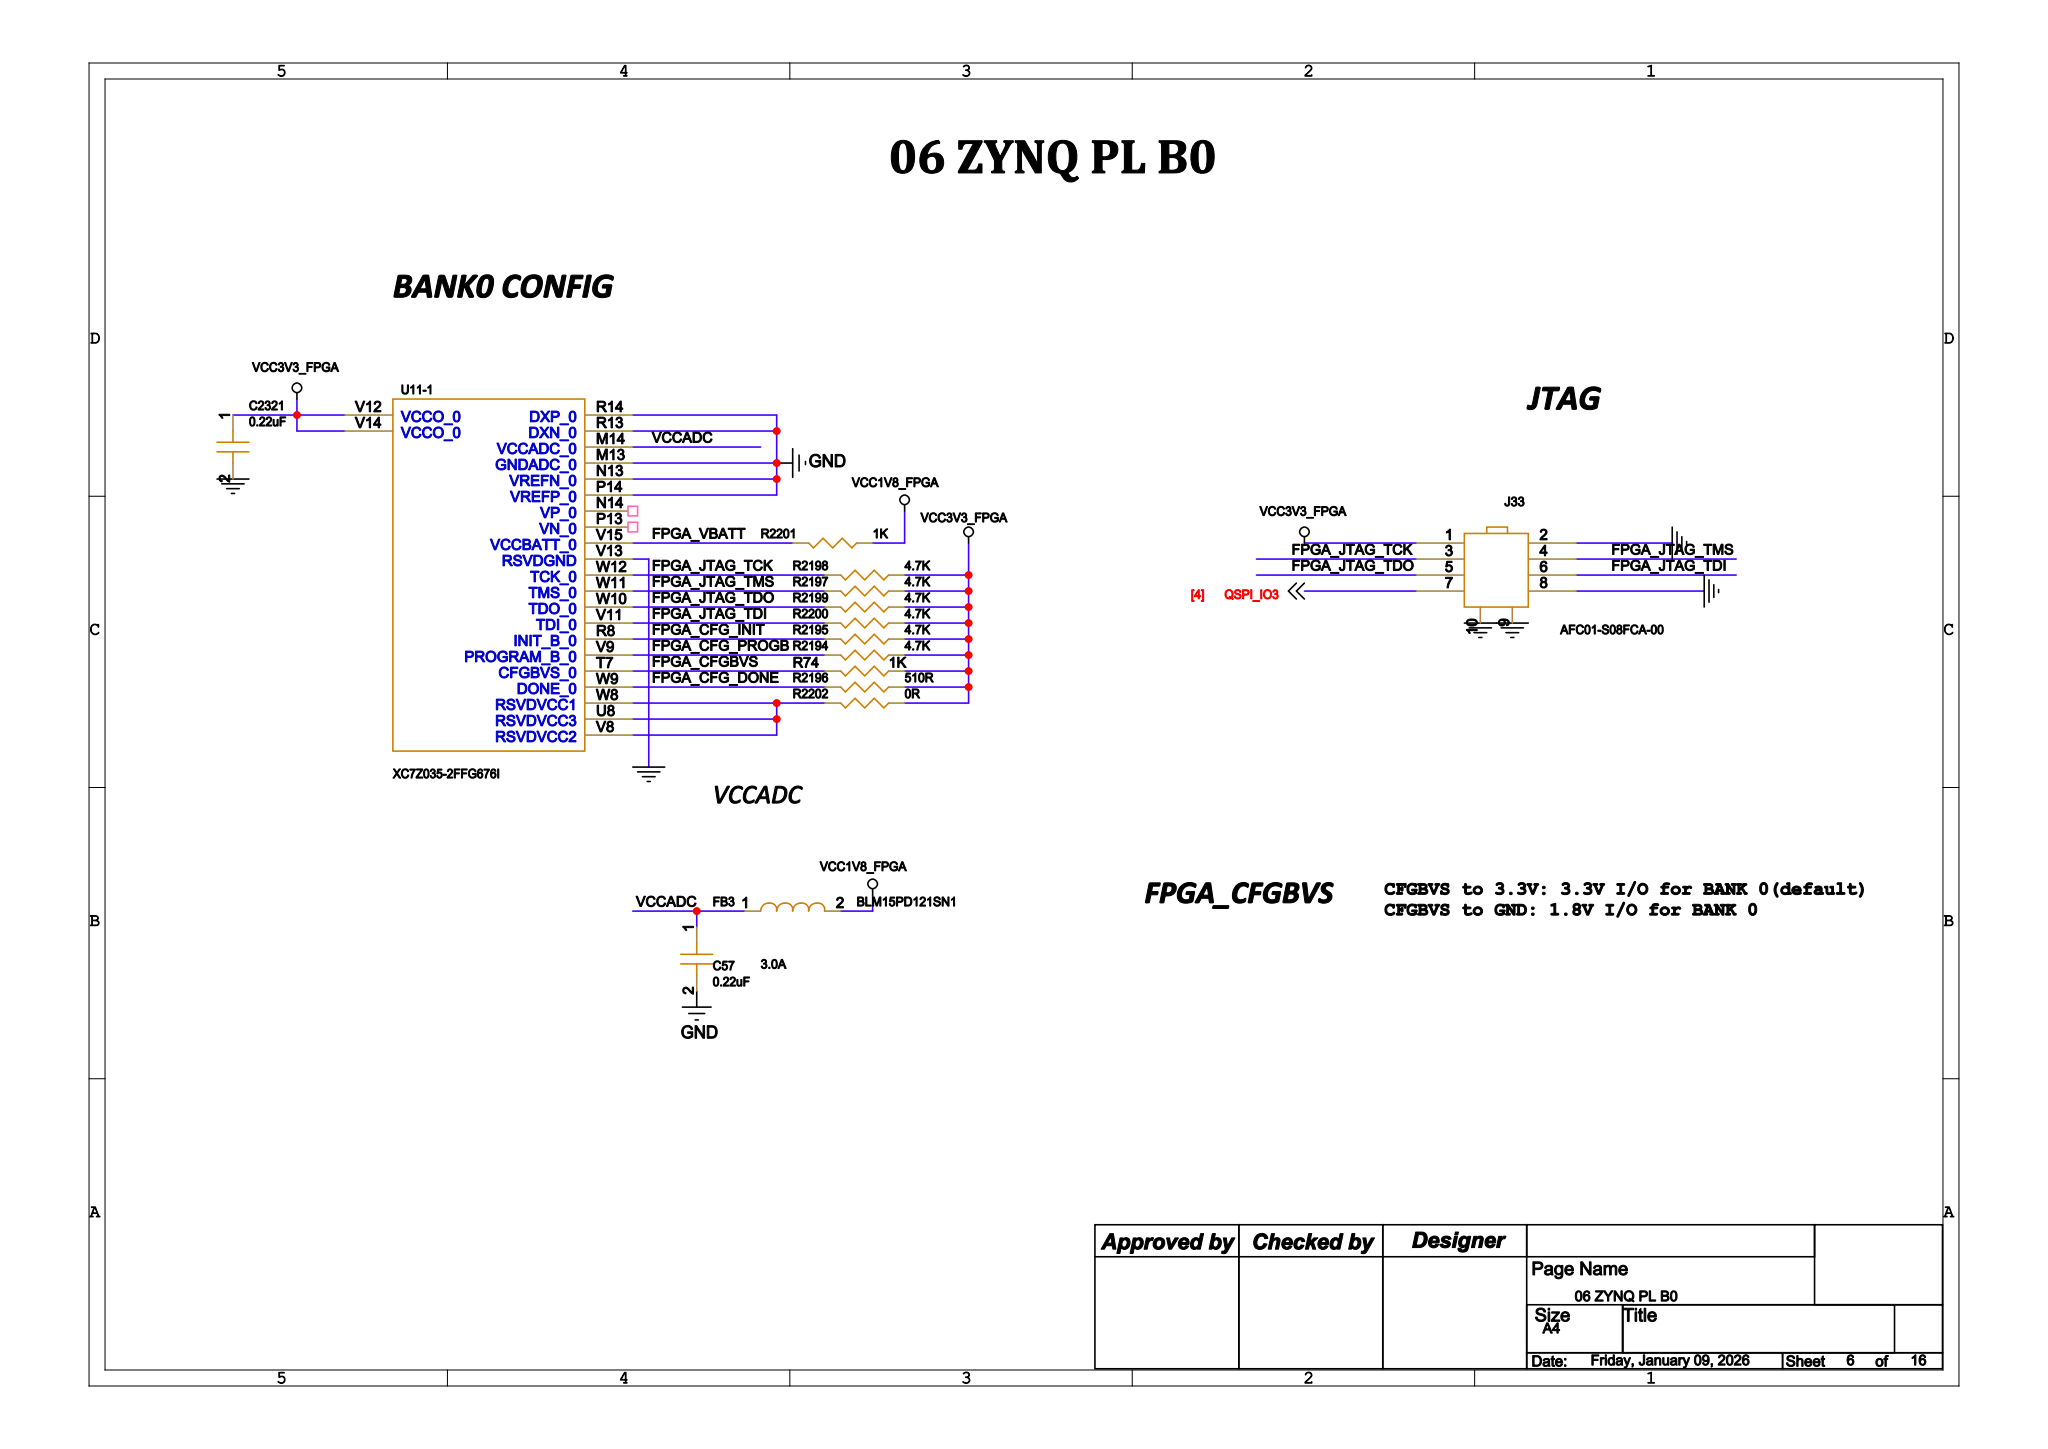Circuit board | Cadence Allegro | 442 parts | 326 nets | one sheet of the schematic
Parts on this sheet (reference | value | footprint):
C57 | 0.22uF | C0201
C2321 | 0.22uF | C0201
FB3 | BLM15PD121SN1 | L0402_D
J33 | AFC01-S08FCA-00 | AFC01-S08FCA-00
R74 | 1K | R0201
R2194 | 4.7K | R0201
R2195 | 4.7K | R0201
R2196 | 510R | R0201
R2197 | 4.7K | R0201
R2198 | 4.7K | R0201
R2199 | 4.7K | R0201
R2200 | 4.7K | R0201
R2201 | 1K | R0201
R2202 | 0R | R0201
Nets of these parts (net: part-pin ...):
GND: C57-2 C2321-2 J33-2 J33-8 J33-9 J33-10
VCC1V8_FPGA: FB3-2 R2201-2
VCC3V3_FPGA: C2321-1 J33-1 R74-2 R2194-2 R2195-2 R2196-2 R2197-2 R2198-2 R2199-2 R2200-2 R2202-2
FPGA_JTAG_TCK: J33-3 R2198-1
FPGA_JTAG_TMS: J33-4 R2197-1
FPGA_JTAG_TDO: J33-5 R2199-1
FPGA_JTAG_TDI: J33-6 R2200-1
QSPI_IO3: J33-7
VCCADC: C57-1 FB3-1
FPGA_CFG_PROGB: R2194-1
FPGA_CFG_INIT: R2195-1
FPGA_CFG_DONE: R2196-1
FPGA_VBATT: R2201-1
N50225355: R2202-1
FPGA_CFGBVS: R74-1